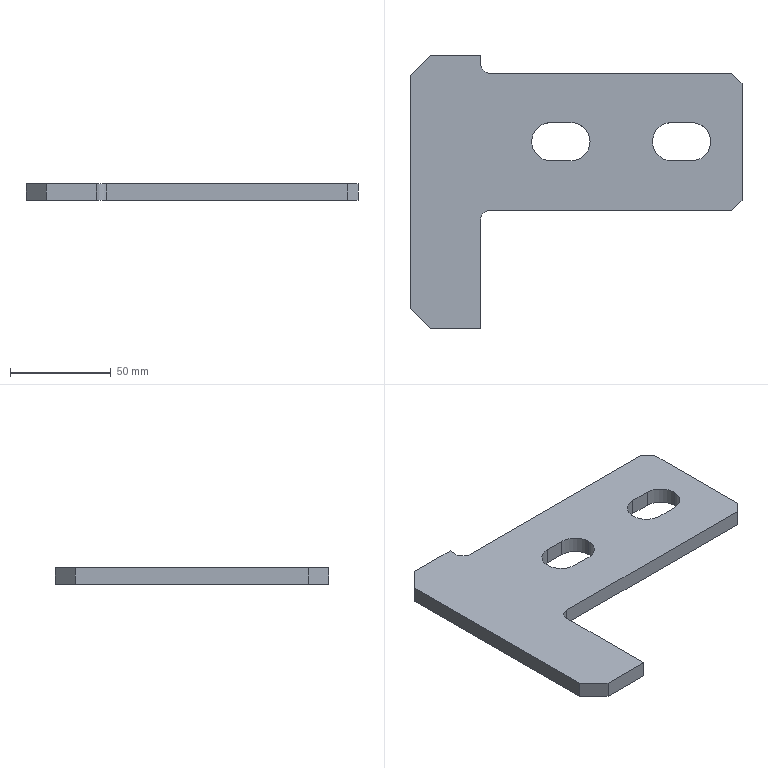Part | STEP file | 筋Plate-150×75-100 | 1 solid | 26 faces | box 165 x 136 x 8 mm | volume 100309 mm3 | plane 18 | cylinder 8 | commonest cylinder face diameters 19 x6 10 x2